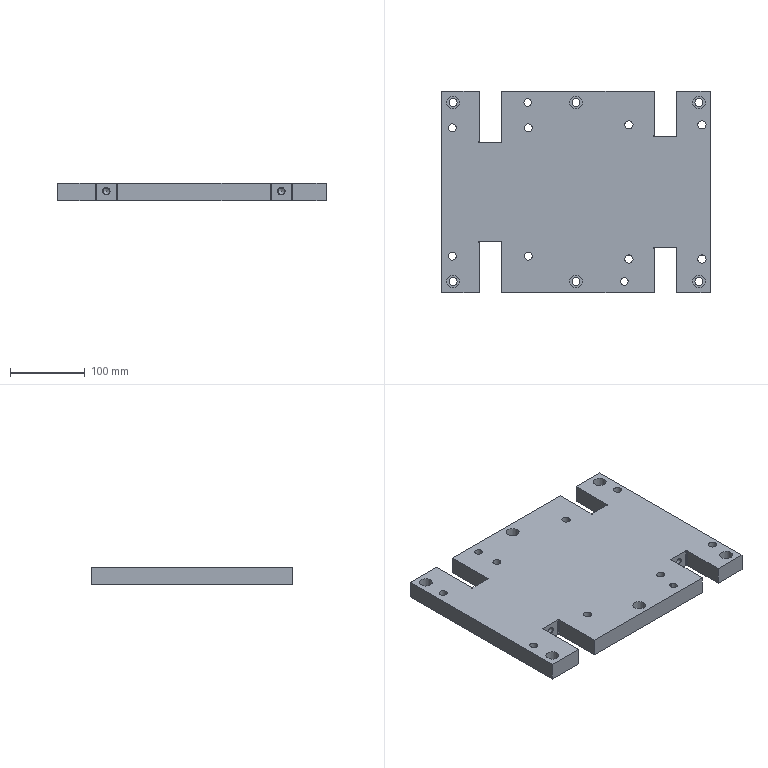Part | STEP file | YBQDJ-YB-1 | 1 solid | 108 faces | box 360 x 270 x 24 mm | volume 2084097 mm3 | cylinder 64 | plane 36 | cone 8 | commonest cylinder face diameters 4 x20 17 x14 1 x10 10.7 x10 8.5 x4 11 x4